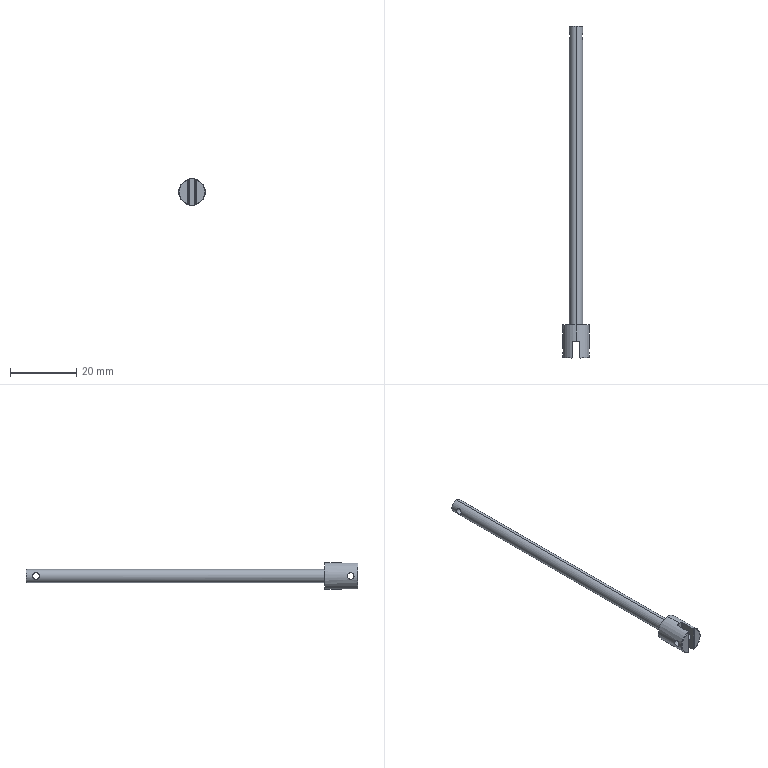Part | SolidWorks | features ICE 4, Fillet 2, Extrusion 1 | 1 solid | 23 faces | box 8 x 100 x 8 mm | volume 1520 mm3 | cylinder 14 | plane 7 | torus 2 | commonest cylinder face diameters 2 x6 0.4 x4 4 x2 8 x2
STEP:
#1=CARTESIAN_POINT('',(-1.732,-3.,1.));
#2=VERTEX_POINT('',#1);
#3=CARTESIAN_POINT('',(-1.732,-3.,-1.));
#4=VERTEX_POINT('',#3);
#5=CARTESIAN_POINT('',(-1.732,-3.,1.));
#6=CARTESIAN_POINT('',(-1.732,-3.066,1.));
#7=CARTESIAN_POINT('',(-1.736,-3.134,0.9932));
#8=CARTESIAN_POINT('',(-1.751,-3.263,0.967));
#9=CARTESIAN_POINT('',(-1.761,-3.326,0.9477));
#10=CARTESIAN_POINT('',(-1.801,-3.508,0.8713));
#11=CARTESIAN_POINT('',(-1.836,-3.616,0.798));
#12=CARTESIAN_POINT('',(-1.905,-3.798,0.6163));
#13=CARTESIAN_POINT('',(-1.939,-3.872,0.5068));
#14=CARTESIAN_POINT('',(-1.986,-3.972,0.2668));
#15=CARTESIAN_POINT('',(-2.,-4.,0.1333));
#16=CARTESIAN_POINT('',(-2.,-4.,-0.1315));
#17=CARTESIAN_POINT('',(-1.986,-3.973,-0.2649));
#18=CARTESIAN_POINT('',(-1.939,-3.872,-0.5074));
#19=CARTESIAN_POINT('',(-1.905,-3.798,-0.6164));
#20=CARTESIAN_POINT('',(-1.836,-3.615,-0.7989));
#21=CARTESIAN_POINT('',(-1.801,-3.507,-0.872));
#22=CARTESIAN_POINT('',(-1.749,-3.267,-0.9726));
#23=CARTESIAN_POINT('',(-1.732,-3.134,-1.));
#24=CARTESIAN_POINT('',(-1.732,-3.,-1.));
#25=B_SPLINE_CURVE_WITH_KNOTS('',3,(#5,#6,#7,#8,#9,#10,#11,#12,#13,#14,#15,#16,#17,#18,#19,#20,#21,#22,#23,#24),.UNSPECIFIED.,.F.,.F.,(4,2,2,2,2,2,2,2,2,4),(0.003181,0.003379,0.003577,0.003974,0.004371,0.004768,0.005165,0.005562,0.005959,0.006356),.UNSPECIFIED.);
#26=EDGE_CURVE('',#2,#4,#25,.T.);
#27=ORIENTED_EDGE('',*,*,#26,.F.);
#28=CARTESIAN_POINT('',(1.732,-3.,1.));
#29=VERTEX_POINT('',#28);
#30=CARTESIAN_POINT('',(-5.,-3.,1.));
#31=DIRECTION('',(1.,0.,0.));
#32=VECTOR('',#31,1000.);
#33=LINE('',#30,#32);
#34=EDGE_CURVE('',#2,#29,#33,.T.);
#35=ORIENTED_EDGE('',*,*,#34,.T.);
#36=CARTESIAN_POINT('',(1.732,-3.,-1.));
#37=VERTEX_POINT('',#36);
#38=CARTESIAN_POINT('',(1.732,-3.,-1.));
#39=CARTESIAN_POINT('',(1.732,-3.135,-1.));
#40=CARTESIAN_POINT('',(1.748,-3.266,-0.9727));
#41=CARTESIAN_POINT('',(1.801,-3.507,-0.8717));
#42=CARTESIAN_POINT('',(1.836,-3.616,-0.798));
#43=CARTESIAN_POINT('',(1.905,-3.798,-0.6167));
#44=CARTESIAN_POINT('',(1.938,-3.872,-0.5072));
#45=CARTESIAN_POINT('',(1.986,-3.973,-0.2669));
#46=CARTESIAN_POINT('',(2.,-4.,-0.1339));
#47=CARTESIAN_POINT('',(2.,-4.,0.1326));
#48=CARTESIAN_POINT('',(1.986,-3.973,0.2658));
#49=CARTESIAN_POINT('',(1.938,-3.871,0.5087));
#50=CARTESIAN_POINT('',(1.905,-3.797,0.6177));
#51=CARTESIAN_POINT('',(1.836,-3.615,0.7989));
#52=CARTESIAN_POINT('',(1.801,-3.506,0.8725));
#53=CARTESIAN_POINT('',(1.748,-3.266,0.9726));
#54=CARTESIAN_POINT('',(1.732,-3.133,1.));
#55=CARTESIAN_POINT('',(1.732,-3.,1.));
#56=B_SPLINE_CURVE_WITH_KNOTS('',3,(#38,#39,#40,#41,#42,#43,#44,#45,#46,#47,#48,#49,#50,#51,#52,#53,#54,#55),.UNSPECIFIED.,.F.,.F.,(4,2,2,2,2,2,2,2,4),(0.,0.0003976,0.0007951,0.001193,0.00159,0.001988,0.002385,0.002783,0.003181),.UNSPECIFIED.);
#57=EDGE_CURVE('',#37,#29,#56,.T.);
#58=ORIENTED_EDGE('',*,*,#57,.F.);
#59=CARTESIAN_POINT('',(-5.,-3.,-1.));
#60=DIRECTION('',(1.,0.,0.));
#61=VECTOR('',#60,1000.);
#62=LINE('',#59,#61);
#63=EDGE_CURVE('',#4,#37,#62,.T.);
#64=ORIENTED_EDGE('',*,*,#63,.F.);
#65=EDGE_LOOP('',(#27,#35,#58,#64));
#66=FACE_OUTER_BOUND('',#65,.T.);
#67=CARTESIAN_POINT('',(-5.,-3.,0.));
#68=DIRECTION('',(1.,0.,0.));
#69=DIRECTION('',(0.,0.,-1.));
#70=AXIS2_PLACEMENT_3D('',#67,#68,#69);
#71=CYLINDRICAL_SURFACE('',#70,1.);
#72=ADVANCED_FACE('',(#66),#71,.F.);
#73=CARTESIAN_POINT('',(-4.,-96.8,0.));
#74=VERTEX_POINT('',#73);
#75=CARTESIAN_POINT('',(-4.,-98.8,0.));
#76=VERTEX_POINT('',#75);
#77=CARTESIAN_POINT('',(-4.,-96.8,0.));
#78=CARTESIAN_POINT('',(-4.,-96.8,-0.1327));
#79=CARTESIAN_POINT('',(-3.993,-96.826,-0.2629));
#80=CARTESIAN_POINT('',(-3.97,-96.927,-0.5049));
#81=CARTESIAN_POINT('',(-3.953,-97.001,-0.6155));
#82=CARTESIAN_POINT('',(-3.92,-97.185,-0.7991));
#83=CARTESIAN_POINT('',(-3.904,-97.296,-0.8735));
#84=CARTESIAN_POINT('',(-3.88,-97.537,-0.9734));
#85=CARTESIAN_POINT('',(-3.873,-97.669,-0.9999));
#86=CARTESIAN_POINT('',(-3.873,-97.931,-1.));
#87=CARTESIAN_POINT('',(-3.88,-98.062,-0.974));
#88=CARTESIAN_POINT('',(-3.904,-98.305,-0.8732));
#89=CARTESIAN_POINT('',(-3.92,-98.415,-0.7996));
#90=CARTESIAN_POINT('',(-3.954,-98.6,-0.6143));
#91=CARTESIAN_POINT('',(-3.97,-98.673,-0.5041));
#92=CARTESIAN_POINT('',(-3.993,-98.774,-0.2626));
#93=CARTESIAN_POINT('',(-4.,-98.8,-0.1308));
#94=CARTESIAN_POINT('',(-4.,-98.8,0.));
#95=B_SPLINE_CURVE_WITH_KNOTS('',3,(#77,#78,#79,#80,#81,#82,#83,#84,#85,#86,#87,#88,#89,#90,#91,#92,#93,#94),.UNSPECIFIED.,.F.,.F.,(4,2,2,2,2,2,2,2,4),(0.,0.0003924,0.0007847,0.001177,0.001569,0.001962,0.002354,0.002747,0.003139),.UNSPECIFIED.);
#96=EDGE_CURVE('',#74,#76,#95,.T.);
#97=ORIENTED_EDGE('',*,*,#96,.T.);
#98=CARTESIAN_POINT('',(-1.05,-98.8,0.));
#99=VERTEX_POINT('',#98);
#100=CARTESIAN_POINT('',(-201.05,-98.8,0.));
#101=DIRECTION('',(1.,0.,0.));
#102=VECTOR('',#101,1000.);
#103=LINE('',#100,#102);
#104=EDGE_CURVE('',#76,#99,#103,.T.);
#105=ORIENTED_EDGE('',*,*,#104,.T.);
#106=CARTESIAN_POINT('',(-1.05,-96.8,0.));
#107=VERTEX_POINT('',#106);
#108=CARTESIAN_POINT('',(-1.05,-97.8,0.));
#109=DIRECTION('',(-1.,0.,0.));
#110=DIRECTION('',(0.,-1.,0.));
#111=AXIS2_PLACEMENT_3D('',#108,#109,#110);
#112=CIRCLE('',#111,1.);
#113=EDGE_CURVE('',#107,#99,#112,.T.);
#114=ORIENTED_EDGE('',*,*,#113,.F.);
#115=CARTESIAN_POINT('',(-201.05,-96.8,0.));
#116=DIRECTION('',(1.,0.,0.));
#117=VECTOR('',#116,1000.);
#118=LINE('',#115,#117);
#119=EDGE_CURVE('',#74,#107,#118,.T.);
#120=ORIENTED_EDGE('',*,*,#119,.F.);
#121=EDGE_LOOP('',(#97,#105,#114,#120));
#122=FACE_OUTER_BOUND('',#121,.T.);
#123=CARTESIAN_POINT('',(-201.05,-97.8,0.));
#124=DIRECTION('',(1.,0.,0.));
#125=DIRECTION('',(0.,1.,0.));
#126=AXIS2_PLACEMENT_3D('',#123,#124,#125);
#127=CYLINDRICAL_SURFACE('',#126,1.);
#128=ADVANCED_FACE('',(#122),#127,.F.);
#129=CARTESIAN_POINT('',(1.05,-98.8,0.));
#130=VERTEX_POINT('',#129);
#131=CARTESIAN_POINT('',(1.05,-96.8,0.));
#132=VERTEX_POINT('',#131);
#133=CARTESIAN_POINT('',(1.05,-97.8,0.));
#134=DIRECTION('',(1.,0.,0.));
#135=DIRECTION('',(0.,1.,0.));
#136=AXIS2_PLACEMENT_3D('',#133,#134,#135);
#137=CIRCLE('',#136,1.);
#138=EDGE_CURVE('',#130,#132,#137,.T.);
#139=ORIENTED_EDGE('',*,*,#138,.F.);
#140=CARTESIAN_POINT('',(4.,-98.8,0.));
#141=VERTEX_POINT('',#140);
#142=CARTESIAN_POINT('',(-201.05,-98.8,0.));
#143=DIRECTION('',(1.,0.,0.));
#144=VECTOR('',#143,1000.);
#145=LINE('',#142,#144);
#146=EDGE_CURVE('',#130,#141,#145,.T.);
#147=ORIENTED_EDGE('',*,*,#146,.T.);
#148=CARTESIAN_POINT('',(4.,-96.8,0.));
#149=VERTEX_POINT('',#148);
#150=CARTESIAN_POINT('',(4.,-98.8,0.));
#151=CARTESIAN_POINT('',(4.,-98.8,-0.1308));
#152=CARTESIAN_POINT('',(3.993,-98.774,-0.2629));
#153=CARTESIAN_POINT('',(3.97,-98.674,-0.5038));
#154=CARTESIAN_POINT('',(3.954,-98.6,-0.6146));
#155=CARTESIAN_POINT('',(3.92,-98.415,-0.7991));
#156=CARTESIAN_POINT('',(3.904,-98.306,-0.8727));
#157=CARTESIAN_POINT('',(3.88,-98.062,-0.9739));
#158=CARTESIAN_POINT('',(3.873,-97.932,-1.));
#159=CARTESIAN_POINT('',(3.873,-97.668,-1.));
#160=CARTESIAN_POINT('',(3.88,-97.537,-0.9737));
#161=CARTESIAN_POINT('',(3.904,-97.296,-0.8736));
#162=CARTESIAN_POINT('',(3.92,-97.185,-0.7992));
#163=CARTESIAN_POINT('',(3.953,-97.001,-0.6158));
#164=CARTESIAN_POINT('',(3.97,-96.927,-0.5048));
#165=CARTESIAN_POINT('',(3.993,-96.827,-0.2641));
#166=CARTESIAN_POINT('',(4.,-96.8,-0.1327));
#167=CARTESIAN_POINT('',(4.,-96.8,0.));
#168=B_SPLINE_CURVE_WITH_KNOTS('',3,(#150,#151,#152,#153,#154,#155,#156,#157,#158,#159,#160,#161,#162,#163,#164,#165,#166,#167),.UNSPECIFIED.,.F.,.F.,(4,2,2,2,2,2,2,2,4),(0.003139,0.003531,0.003923,0.004316,0.004708,0.0051,0.005493,0.005885,0.006277),.UNSPECIFIED.);
#169=EDGE_CURVE('',#141,#149,#168,.T.);
#170=ORIENTED_EDGE('',*,*,#169,.T.);
#171=CARTESIAN_POINT('',(-201.05,-96.8,0.));
#172=DIRECTION('',(1.,0.,0.));
#173=VECTOR('',#172,1000.);
#174=LINE('',#171,#173);
#175=EDGE_CURVE('',#132,#149,#174,.T.);
#176=ORIENTED_EDGE('',*,*,#175,.F.);
#177=EDGE_LOOP('',(#139,#147,#170,#176));
#178=FACE_OUTER_BOUND('',#177,.T.);
#179=CARTESIAN_POINT('',(-201.05,-97.8,0.));
#180=DIRECTION('',(1.,0.,0.));
#181=DIRECTION('',(0.,1.,0.));
#182=AXIS2_PLACEMENT_3D('',#179,#180,#181);
#183=CYLINDRICAL_SURFACE('',#182,1.);
#184=ADVANCED_FACE('',(#178),#183,.F.);
#185=CARTESIAN_POINT('',(4.,-96.8,0.));
#186=CARTESIAN_POINT('',(4.,-96.8,0.1327));
#187=CARTESIAN_POINT('',(3.993,-96.826,0.2629));
#188=CARTESIAN_POINT('',(3.97,-96.927,0.5049));
#189=CARTESIAN_POINT('',(3.953,-97.001,0.6155));
#190=CARTESIAN_POINT('',(3.92,-97.185,0.7991));
#191=CARTESIAN_POINT('',(3.904,-97.296,0.8735));
#192=CARTESIAN_POINT('',(3.88,-97.537,0.9734));
#193=CARTESIAN_POINT('',(3.873,-97.669,0.9999));
#194=CARTESIAN_POINT('',(3.873,-97.931,1.));
#195=CARTESIAN_POINT('',(3.88,-98.062,0.974));
#196=CARTESIAN_POINT('',(3.904,-98.305,0.8732));
#197=CARTESIAN_POINT('',(3.92,-98.415,0.7996));
#198=CARTESIAN_POINT('',(3.954,-98.6,0.6143));
#199=CARTESIAN_POINT('',(3.97,-98.673,0.5041));
#200=CARTESIAN_POINT('',(3.993,-98.774,0.2626));
#201=CARTESIAN_POINT('',(4.,-98.8,0.1308));
#202=CARTESIAN_POINT('',(4.,-98.8,0.));
#203=B_SPLINE_CURVE_WITH_KNOTS('',3,(#185,#186,#187,#188,#189,#190,#191,#192,#193,#194,#195,#196,#197,#198,#199,#200,#201,#202),.UNSPECIFIED.,.F.,.F.,(4,2,2,2,2,2,2,2,4),(0.,0.0003924,0.0007847,0.001177,0.001569,0.001962,0.002354,0.002747,0.003139),.UNSPECIFIED.);
#204=EDGE_CURVE('',#149,#141,#203,.T.);
#205=ORIENTED_EDGE('',*,*,#204,.F.);
#206=ORIENTED_EDGE('',*,*,#169,.F.);
#207=EDGE_LOOP('',(#205,#206));
#208=FACE_BOUND('',#207,.T.);
#209=CARTESIAN_POINT('',(0.,-90.,-4.));
#210=VERTEX_POINT('',#209);
#211=CARTESIAN_POINT('',(0.,-90.,4.));
#212=VERTEX_POINT('',#211);
#213=CARTESIAN_POINT('',(0.,-90.,0.));
#214=DIRECTION('',(0.,-1.,0.));
#215=DIRECTION('',(0.,0.,-1.));
#216=AXIS2_PLACEMENT_3D('',#213,#214,#215);
#217=CIRCLE('',#216,4.);
#218=EDGE_CURVE('',#210,#212,#217,.T.);
#219=ORIENTED_EDGE('',*,*,#218,.T.);
#220=CARTESIAN_POINT('',(0.,-95.,4.));
#221=VERTEX_POINT('',#220);
#222=CARTESIAN_POINT('',(0.,-90.,4.));
#223=DIRECTION('',(0.,-1.,0.));
#224=VECTOR('',#223,1000.);
#225=LINE('',#222,#224);
#226=EDGE_CURVE('',#212,#221,#225,.T.);
#227=ORIENTED_EDGE('',*,*,#226,.T.);
#228=CARTESIAN_POINT('',(0.85,-95.,3.909));
#229=VERTEX_POINT('',#228);
#230=CARTESIAN_POINT('',(0.,-95.,0.));
#231=DIRECTION('',(0.,-1.,0.));
#232=DIRECTION('',(0.,0.,1.));
#233=AXIS2_PLACEMENT_3D('',#230,#231,#232);
#234=CIRCLE('',#233,4.);
#235=EDGE_CURVE('',#229,#221,#234,.T.);
#236=ORIENTED_EDGE('',*,*,#235,.F.);
#237=CARTESIAN_POINT('',(1.05,-95.2,3.86));
#238=VERTEX_POINT('',#237);
#239=CARTESIAN_POINT('',(0.85,-95.,3.909));
#240=CARTESIAN_POINT('',(0.9024,-95.,3.897));
#241=CARTESIAN_POINT('',(0.9534,-95.021,3.885));
#242=CARTESIAN_POINT('',(1.028,-95.094,3.866));
#243=CARTESIAN_POINT('',(1.05,-95.146,3.86));
#244=CARTESIAN_POINT('',(1.05,-95.2,3.86));
#245=B_SPLINE_CURVE_WITH_KNOTS('',3,(#239,#240,#241,#242,#243,#244),.UNSPECIFIED.,.F.,.F.,(4,2,4),(0.,0.0001585,0.0003169),.UNSPECIFIED.);
#246=EDGE_CURVE('',#229,#238,#245,.T.);
#247=ORIENTED_EDGE('',*,*,#246,.T.);
#248=CARTESIAN_POINT('',(1.05,-99.8,3.86));
#249=VERTEX_POINT('',#248);
#250=CARTESIAN_POINT('',(1.05,-90.,3.86));
#251=DIRECTION('',(0.,1.,0.));
#252=VECTOR('',#251,1000.);
#253=LINE('',#250,#252);
#254=EDGE_CURVE('',#249,#238,#253,.T.);
#255=ORIENTED_EDGE('',*,*,#254,.F.);
#256=CARTESIAN_POINT('',(1.05,-99.8,-3.86));
#257=VERTEX_POINT('',#256);
#258=CARTESIAN_POINT('',(0.,-99.8,0.));
#259=DIRECTION('',(0.,1.,0.));
#260=DIRECTION('',(0.,0.,-1.));
#261=AXIS2_PLACEMENT_3D('',#258,#259,#260);
#262=CIRCLE('',#261,4.);
#263=EDGE_CURVE('',#249,#257,#262,.T.);
#264=ORIENTED_EDGE('',*,*,#263,.T.);
#265=CARTESIAN_POINT('',(1.05,-95.2,-3.86));
#266=VERTEX_POINT('',#265);
#267=CARTESIAN_POINT('',(1.05,-90.,-3.86));
#268=DIRECTION('',(0.,-1.,0.));
#269=VECTOR('',#268,1000.);
#270=LINE('',#267,#269);
#271=EDGE_CURVE('',#266,#257,#270,.T.);
#272=ORIENTED_EDGE('',*,*,#271,.F.);
#273=CARTESIAN_POINT('',(0.85,-95.,-3.909));
#274=VERTEX_POINT('',#273);
#275=CARTESIAN_POINT('',(1.05,-95.2,-3.86));
#276=CARTESIAN_POINT('',(1.05,-95.146,-3.86));
#277=CARTESIAN_POINT('',(1.028,-95.094,-3.866));
#278=CARTESIAN_POINT('',(0.9536,-95.021,-3.885));
#279=CARTESIAN_POINT('',(0.9023,-95.,-3.897));
#280=CARTESIAN_POINT('',(0.85,-95.,-3.909));
#281=B_SPLINE_CURVE_WITH_KNOTS('',3,(#275,#276,#277,#278,#279,#280),.UNSPECIFIED.,.F.,.F.,(4,2,4),(0.,0.0001585,0.0003169),.UNSPECIFIED.);
#282=EDGE_CURVE('',#266,#274,#281,.T.);
#283=ORIENTED_EDGE('',*,*,#282,.T.);
#284=CARTESIAN_POINT('',(0.,-95.,-4.));
#285=VERTEX_POINT('',#284);
#286=CARTESIAN_POINT('',(0.,-95.,0.));
#287=DIRECTION('',(0.,-1.,0.));
#288=DIRECTION('',(0.,0.,1.));
#289=AXIS2_PLACEMENT_3D('',#286,#287,#288);
#290=CIRCLE('',#289,4.);
#291=EDGE_CURVE('',#285,#274,#290,.T.);
#292=ORIENTED_EDGE('',*,*,#291,.F.);
#293=CARTESIAN_POINT('',(0.,-90.,-4.));
#294=DIRECTION('',(0.,-1.,0.));
#295=VECTOR('',#294,1000.);
#296=LINE('',#293,#295);
#297=EDGE_CURVE('',#210,#285,#296,.T.);
#298=ORIENTED_EDGE('',*,*,#297,.F.);
#299=EDGE_LOOP('',(#219,#227,#236,#247,#255,#264,#272,#283,#292,#298));
#300=FACE_OUTER_BOUND('',#299,.T.);
#301=CARTESIAN_POINT('',(0.,-90.,0.));
#302=DIRECTION('',(0.,-1.,0.));
#303=DIRECTION('',(0.,0.,-1.));
#304=AXIS2_PLACEMENT_3D('',#301,#302,#303);
#305=CYLINDRICAL_SURFACE('',#304,4.);
#306=ADVANCED_FACE('',(#208,#300),#305,.T.);
#307=ORIENTED_EDGE('',*,*,#57,.T.);
#308=CARTESIAN_POINT('',(1.732,-3.,1.));
#309=CARTESIAN_POINT('',(1.732,-2.934,1.));
#310=CARTESIAN_POINT('',(1.736,-2.866,0.9932));
#311=CARTESIAN_POINT('',(1.751,-2.737,0.967));
#312=CARTESIAN_POINT('',(1.761,-2.674,0.9477));
#313=CARTESIAN_POINT('',(1.801,-2.492,0.8713));
#314=CARTESIAN_POINT('',(1.836,-2.384,0.798));
#315=CARTESIAN_POINT('',(1.905,-2.202,0.6163));
#316=CARTESIAN_POINT('',(1.939,-2.128,0.5068));
#317=CARTESIAN_POINT('',(1.986,-2.028,0.2668));
#318=CARTESIAN_POINT('',(2.,-2.,0.1333));
#319=CARTESIAN_POINT('',(2.,-2.,-0.1315));
#320=CARTESIAN_POINT('',(1.986,-2.027,-0.2649));
#321=CARTESIAN_POINT('',(1.939,-2.128,-0.5074));
#322=CARTESIAN_POINT('',(1.905,-2.202,-0.6164));
#323=CARTESIAN_POINT('',(1.836,-2.385,-0.7989));
#324=CARTESIAN_POINT('',(1.801,-2.493,-0.872));
#325=CARTESIAN_POINT('',(1.749,-2.733,-0.9726));
#326=CARTESIAN_POINT('',(1.732,-2.866,-1.));
#327=CARTESIAN_POINT('',(1.732,-3.,-1.));
#328=B_SPLINE_CURVE_WITH_KNOTS('',3,(#308,#309,#310,#311,#312,#313,#314,#315,#316,#317,#318,#319,#320,#321,#322,#323,#324,#325,#326,#327),.UNSPECIFIED.,.F.,.F.,(4,2,2,2,2,2,2,2,2,4),(0.003181,0.003379,0.003577,0.003974,0.004371,0.004768,0.005165,0.005562,0.005959,0.006356),.UNSPECIFIED.);
#329=EDGE_CURVE('',#29,#37,#328,.T.);
#330=ORIENTED_EDGE('',*,*,#329,.T.);
#331=EDGE_LOOP('',(#307,#330));
#332=FACE_BOUND('',#331,.T.);
#333=CARTESIAN_POINT('',(0.,-90.,-2.));
#334=VERTEX_POINT('',#333);
#335=CARTESIAN_POINT('',(0.,-90.,2.));
#336=VERTEX_POINT('',#335);
#337=CARTESIAN_POINT('',(0.,-90.,0.));
#338=DIRECTION('',(0.,-1.,0.));
#339=DIRECTION('',(0.,0.,-1.));
#340=AXIS2_PLACEMENT_3D('',#337,#338,#339);
#341=CIRCLE('',#340,2.);
#342=EDGE_CURVE('',#334,#336,#341,.T.);
#343=ORIENTED_EDGE('',*,*,#342,.F.);
#344=CARTESIAN_POINT('',(0.,0.,-2.));
#345=VERTEX_POINT('',#344);
#346=CARTESIAN_POINT('',(0.,-100.,-2.));
#347=DIRECTION('',(0.,1.,0.));
#348=VECTOR('',#347,1000.);
#349=LINE('',#346,#348);
#350=EDGE_CURVE('',#334,#345,#349,.T.);
#351=ORIENTED_EDGE('',*,*,#350,.T.);
#352=CARTESIAN_POINT('',(0.,0.,2.));
#353=VERTEX_POINT('',#352);
#354=CARTESIAN_POINT('',(0.,0.,0.));
#355=DIRECTION('',(0.,-1.,0.));
#356=DIRECTION('',(0.,0.,-1.));
#357=AXIS2_PLACEMENT_3D('',#354,#355,#356);
#358=CIRCLE('',#357,2.);
#359=EDGE_CURVE('',#345,#353,#358,.T.);
#360=ORIENTED_EDGE('',*,*,#359,.T.);
#361=CARTESIAN_POINT('',(0.,-100.,2.));
#362=DIRECTION('',(0.,1.,0.));
#363=VECTOR('',#362,1000.);
#364=LINE('',#361,#363);
#365=EDGE_CURVE('',#336,#353,#364,.T.);
#366=ORIENTED_EDGE('',*,*,#365,.F.);
#367=EDGE_LOOP('',(#343,#351,#360,#366));
#368=FACE_OUTER_BOUND('',#367,.T.);
#369=CARTESIAN_POINT('',(0.,-100.,0.));
#370=DIRECTION('',(0.,1.,0.));
#371=DIRECTION('',(0.,0.,1.));
#372=AXIS2_PLACEMENT_3D('',#369,#370,#371);
#373=CYLINDRICAL_SURFACE('',#372,2.);
#374=ADVANCED_FACE('',(#332,#368),#373,.T.);
#375=CARTESIAN_POINT('',(-1.25,-100.,-3.589));
#376=VERTEX_POINT('',#375);
#377=CARTESIAN_POINT('',(-1.25,-100.,3.589));
#378=VERTEX_POINT('',#377);
#379=CARTESIAN_POINT('',(-1.25,-100.,3.86));
#380=DIRECTION('',(0.,0.,1.));
#381=VECTOR('',#380,1000.);
#382=LINE('',#379,#381);
#383=EDGE_CURVE('',#376,#378,#382,.T.);
#384=ORIENTED_EDGE('',*,*,#383,.T.);
#385=CARTESIAN_POINT('',(0.,-100.,0.));
#386=DIRECTION('',(0.,-1.,0.));
#387=DIRECTION('',(0.,0.,-1.));
#388=AXIS2_PLACEMENT_3D('',#385,#386,#387);
#389=CIRCLE('',#388,3.8);
#390=EDGE_CURVE('',#378,#376,#389,.T.);
#391=ORIENTED_EDGE('',*,*,#390,.T.);
#392=EDGE_LOOP('',(#384,#391));
#393=FACE_OUTER_BOUND('',#392,.T.);
#394=CARTESIAN_POINT('',(0.,-100.,0.));
#395=DIRECTION('',(0.,-1.,0.));
#396=DIRECTION('',(0.,0.,-1.));
#397=AXIS2_PLACEMENT_3D('',#394,#395,#396);
#398=PLANE('',#397);
#399=ADVANCED_FACE('',(#393),#398,.T.);
#400=ORIENTED_EDGE('',*,*,#350,.F.);
#401=CARTESIAN_POINT('',(0.,-90.,0.));
#402=DIRECTION('',(0.,-1.,0.));
#403=DIRECTION('',(0.,0.,-1.));
#404=AXIS2_PLACEMENT_3D('',#401,#402,#403);
#405=CIRCLE('',#404,2.);
#406=EDGE_CURVE('',#336,#334,#405,.T.);
#407=ORIENTED_EDGE('',*,*,#406,.F.);
#408=ORIENTED_EDGE('',*,*,#365,.T.);
#409=CARTESIAN_POINT('',(0.,0.,0.));
#410=DIRECTION('',(0.,-1.,0.));
#411=DIRECTION('',(0.,0.,-1.));
#412=AXIS2_PLACEMENT_3D('',#409,#410,#411);
#413=CIRCLE('',#412,2.);
#414=EDGE_CURVE('',#353,#345,#413,.T.);
#415=ORIENTED_EDGE('',*,*,#414,.T.);
#416=EDGE_LOOP('',(#400,#407,#408,#415));
#417=FACE_OUTER_BOUND('',#416,.T.);
#418=CARTESIAN_POINT('',(-1.732,-3.,-1.));
#419=CARTESIAN_POINT('',(-1.732,-2.865,-1.));
#420=CARTESIAN_POINT('',(-1.748,-2.734,-0.9727));
#421=CARTESIAN_POINT('',(-1.801,-2.493,-0.8717));
#422=CARTESIAN_POINT('',(-1.836,-2.384,-0.798));
#423=CARTESIAN_POINT('',(-1.905,-2.202,-0.6167));
#424=CARTESIAN_POINT('',(-1.938,-2.128,-0.5072));
#425=CARTESIAN_POINT('',(-1.986,-2.027,-0.2669));
#426=CARTESIAN_POINT('',(-2.,-2.,-0.1339));
#427=CARTESIAN_POINT('',(-2.,-2.,0.1326));
#428=CARTESIAN_POINT('',(-1.986,-2.027,0.2658));
#429=CARTESIAN_POINT('',(-1.938,-2.129,0.5087));
#430=CARTESIAN_POINT('',(-1.905,-2.203,0.6177));
#431=CARTESIAN_POINT('',(-1.836,-2.385,0.7989));
#432=CARTESIAN_POINT('',(-1.801,-2.494,0.8725));
#433=CARTESIAN_POINT('',(-1.748,-2.734,0.9726));
#434=CARTESIAN_POINT('',(-1.732,-2.867,1.));
#435=CARTESIAN_POINT('',(-1.732,-3.,1.));
#436=B_SPLINE_CURVE_WITH_KNOTS('',3,(#418,#419,#420,#421,#422,#423,#424,#425,#426,#427,#428,#429,#430,#431,#432,#433,#434,#435),.UNSPECIFIED.,.F.,.F.,(4,2,2,2,2,2,2,2,4),(0.,0.0003976,0.0007951,0.001193,0.00159,0.001988,0.002385,0.002783,0.003181),.UNSPECIFIED.);
#437=EDGE_CURVE('',#4,#2,#436,.T.);
#438=ORIENTED_EDGE('',*,*,#437,.T.);
#439=ORIENTED_EDGE('',*,*,#26,.T.);
#440=EDGE_LOOP('',(#438,#439));
#441=FACE_BOUND('',#440,.T.);
#442=CARTESIAN_POINT('',(0.,-100.,0.));
#443=DIRECTION('',(0.,1.,0.));
#444=DIRECTION('',(0.,0.,1.));
#445=AXIS2_PLACEMENT_3D('',#442,#443,#444);
#446=CYLINDRICAL_SURFACE('',#445,2.);
#447=ADVANCED_FACE('',(#417,#441),#446,.T.);
#448=ORIENTED_EDGE('',*,*,#414,.F.);
#449=ORIENTED_EDGE('',*,*,#359,.F.);
#450=EDGE_LOOP('',(#448,#449));
#451=FACE_OUTER_BOUND('',#450,.T.);
#452=CARTESIAN_POINT('',(0.,0.,0.));
#453=DIRECTION('',(0.,-1.,0.));
#454=DIRECTION('',(0.,0.,-1.));
#455=AXIS2_PLACEMENT_3D('',#452,#453,#454);
#456=PLANE('',#455);
#457=ADVANCED_FACE('',(#451),#456,.F.);
#458=ORIENTED_EDGE('',*,*,#226,.F.);
#459=CARTESIAN_POINT('',(0.,-90.,0.));
#460=DIRECTION('',(0.,-1.,0.));
#461=DIRECTION('',(0.,0.,-1.));
#462=AXIS2_PLACEMENT_3D('',#459,#460,#461);
#463=CIRCLE('',#462,4.);
#464=EDGE_CURVE('',#212,#210,#463,.T.);
#465=ORIENTED_EDGE('',*,*,#464,.T.);
#466=ORIENTED_EDGE('',*,*,#297,.T.);
#467=CARTESIAN_POINT('',(-0.85,-95.,-3.909));
#468=VERTEX_POINT('',#467);
#469=CARTESIAN_POINT('',(0.,-95.,0.));
#470=DIRECTION('',(0.,-1.,0.));
#471=DIRECTION('',(0.,0.,1.));
#472=AXIS2_PLACEMENT_3D('',#469,#470,#471);
#473=CIRCLE('',#472,4.);
#474=EDGE_CURVE('',#468,#285,#473,.T.);
#475=ORIENTED_EDGE('',*,*,#474,.F.);
#476=CARTESIAN_POINT('',(-1.05,-95.2,-3.86));
#477=VERTEX_POINT('',#476);
#478=CARTESIAN_POINT('',(-0.85,-95.,-3.909));
#479=CARTESIAN_POINT('',(-0.9024,-95.,-3.897));
#480=CARTESIAN_POINT('',(-0.9534,-95.021,-3.885));
#481=CARTESIAN_POINT('',(-1.028,-95.094,-3.866));
#482=CARTESIAN_POINT('',(-1.05,-95.146,-3.86));
#483=CARTESIAN_POINT('',(-1.05,-95.2,-3.86));
#484=B_SPLINE_CURVE_WITH_KNOTS('',3,(#478,#479,#480,#481,#482,#483),.UNSPECIFIED.,.F.,.F.,(4,2,4),(0.,0.0001585,0.0003169),.UNSPECIFIED.);
#485=EDGE_CURVE('',#468,#477,#484,.T.);
#486=ORIENTED_EDGE('',*,*,#485,.T.);
#487=CARTESIAN_POINT('',(-1.05,-99.8,-3.86));
#488=VERTEX_POINT('',#487);
#489=CARTESIAN_POINT('',(-1.05,-90.,-3.86));
#490=DIRECTION('',(0.,1.,0.));
#491=VECTOR('',#490,1000.);
#492=LINE('',#489,#491);
#493=EDGE_CURVE('',#488,#477,#492,.T.);
#494=ORIENTED_EDGE('',*,*,#493,.F.);
#495=CARTESIAN_POINT('',(-1.05,-99.8,3.86));
#496=VERTEX_POINT('',#495);
#497=CARTESIAN_POINT('',(0.,-99.8,0.));
#498=DIRECTION('',(0.,1.,0.));
#499=DIRECTION('',(0.,0.,-1.));
#500=AXIS2_PLACEMENT_3D('',#497,#498,#499);
#501=CIRCLE('',#500,4.);
#502=EDGE_CURVE('',#488,#496,#501,.T.);
#503=ORIENTED_EDGE('',*,*,#502,.T.);
#504=CARTESIAN_POINT('',(-1.05,-95.2,3.86));
#505=VERTEX_POINT('',#504);
#506=CARTESIAN_POINT('',(-1.05,-90.,3.86));
#507=DIRECTION('',(0.,-1.,0.));
#508=VECTOR('',#507,1000.);
#509=LINE('',#506,#508);
#510=EDGE_CURVE('',#505,#496,#509,.T.);
#511=ORIENTED_EDGE('',*,*,#510,.F.);
#512=CARTESIAN_POINT('',(-0.85,-95.,3.909));
#513=VERTEX_POINT('',#512);
#514=CARTESIAN_POINT('',(-1.05,-95.2,3.86));
#515=CARTESIAN_POINT('',(-1.05,-95.146,3.86));
#516=CARTESIAN_POINT('',(-1.028,-95.094,3.866));
#517=CARTESIAN_POINT('',(-0.9536,-95.021,3.885));
#518=CARTESIAN_POINT('',(-0.9023,-95.,3.897));
#519=CARTESIAN_POINT('',(-0.85,-95.,3.909));
#520=B_SPLINE_CURVE_WITH_KNOTS('',3,(#514,#515,#516,#517,#518,#519),.UNSPECIFIED.,.F.,.F.,(4,2,4),(0.,0.0001585,0.0003169),.UNSPECIFIED.);
#521=EDGE_CURVE('',#505,#513,#520,.T.);
#522=ORIENTED_EDGE('',*,*,#521,.T.);
#523=CARTESIAN_POINT('',(0.,-95.,0.));
#524=DIRECTION('',(0.,-1.,0.));
#525=DIRECTION('',(0.,0.,1.));
#526=AXIS2_PLACEMENT_3D('',#523,#524,#525);
#527=CIRCLE('',#526,4.);
#528=EDGE_CURVE('',#221,#513,#527,.T.);
#529=ORIENTED_EDGE('',*,*,#528,.F.);
#530=EDGE_LOOP('',(#458,#465,#466,#475,#486,#494,#503,#511,#522,#529));
#531=FACE_OUTER_BOUND('',#530,.T.);
#532=ORIENTED_EDGE('',*,*,#96,.F.);
#533=CARTESIAN_POINT('',(-4.,-98.8,0.));
#534=CARTESIAN_POINT('',(-4.,-98.8,0.1308));
#535=CARTESIAN_POINT('',(-3.993,-98.774,0.2629));
#536=CARTESIAN_POINT('',(-3.97,-98.674,0.5038));
#537=CARTESIAN_POINT('',(-3.954,-98.6,0.6146));
#538=CARTESIAN_POINT('',(-3.92,-98.415,0.7991));
#539=CARTESIAN_POINT('',(-3.904,-98.306,0.8727));
#540=CARTESIAN_POINT('',(-3.88,-98.062,0.9739));
#541=CARTESIAN_POINT('',(-3.873,-97.932,1.));
#542=CARTESIAN_POINT('',(-3.873,-97.668,1.));
#543=CARTESIAN_POINT('',(-3.88,-97.537,0.9737));
#544=CARTESIAN_POINT('',(-3.904,-97.296,0.8736));
#545=CARTESIAN_POINT('',(-3.92,-97.185,0.7992));
#546=CARTESIAN_POINT('',(-3.953,-97.001,0.6158));
#547=CARTESIAN_POINT('',(-3.97,-96.927,0.5048));
#548=CARTESIAN_POINT('',(-3.993,-96.827,0.2641));
#549=CARTESIAN_POINT('',(-4.,-96.8,0.1327));
#550=CARTESIAN_POINT('',(-4.,-96.8,0.));
#551=B_SPLINE_CURVE_WITH_KNOTS('',3,(#533,#534,#535,#536,#537,#538,#539,#540,#541,#542,#543,#544,#545,#546,#547,#548,#549,#550),.UNSPECIFIED.,.F.,.F.,(4,2,2,2,2,2,2,2,4),(0.003139,0.003531,0.003923,0.004316,0.004708,0.0051,0.005493,0.005885,0.006277),.UNSPECIFIED.);
#552=EDGE_CURVE('',#76,#74,#551,.T.);
#553=ORIENTED_EDGE('',*,*,#552,.F.);
#554=EDGE_LOOP('',(#532,#553));
#555=FACE_BOUND('',#554,.T.);
#556=CARTESIAN_POINT('',(0.,-90.,0.));
#557=DIRECTION('',(0.,-1.,0.));
#558=DIRECTION('',(0.,0.,-1.));
#559=AXIS2_PLACEMENT_3D('',#556,#557,#558);
#560=CYLINDRICAL_SURFACE('',#559,4.);
#561=ADVANCED_FACE('',(#531,#555),#560,.T.);
#562=ORIENTED_EDGE('',*,*,#406,.T.);
#563=ORIENTED_EDGE('',*,*,#342,.T.);
#564=EDGE_LOOP('',(#562,#563));
#565=FACE_BOUND('',#564,.T.);
#566=ORIENTED_EDGE('',*,*,#218,.F.);
#567=ORIENTED_EDGE('',*,*,#464,.F.);
#568=EDGE_LOOP('',(#566,#567));
#569=FACE_OUTER_BOUND('',#568,.T.);
#570=CARTESIAN_POINT('',(0.,-90.,0.));
#571=DIRECTION('',(0.,-1.,0.));
#572=DIRECTION('',(0.,0.,-1.));
#573=AXIS2_PLACEMENT_3D('',#570,#571,#572);
#574=PLANE('',#573);
#575=ADVANCED_FACE('',(#565,#569),#574,.F.);
#576=CARTESIAN_POINT('',(1.25,-100.,3.589));
#577=VERTEX_POINT('',#576);
#578=CARTESIAN_POINT('',(1.25,-100.,-3.589));
#579=VERTEX_POINT('',#578);
#580=CARTESIAN_POINT('',(1.25,-100.,-3.86));
#581=DIRECTION('',(0.,0.,-1.));
#582=VECTOR('',#581,1000.);
#583=LINE('',#580,#582);
#584=EDGE_CURVE('',#577,#579,#583,.T.);
#585=ORIENTED_EDGE('',*,*,#584,.T.);
#586=CARTESIAN_POINT('',(0.,-100.,0.));
#587=DIRECTION('',(0.,-1.,0.));
#588=DIRECTION('',(0.,0.,-1.));
#589=AXIS2_PLACEMENT_3D('',#586,#587,#588);
#590=CIRCLE('',#589,3.8);
#591=EDGE_CURVE('',#579,#577,#590,.T.);
#592=ORIENTED_EDGE('',*,*,#591,.T.);
#593=EDGE_LOOP('',(#585,#592));
#594=FACE_OUTER_BOUND('',#593,.T.);
#595=CARTESIAN_POINT('',(0.,-100.,0.));
#596=DIRECTION('',(0.,-1.,0.));
#597=DIRECTION('',(0.,0.,-1.));
#598=AXIS2_PLACEMENT_3D('',#595,#596,#597);
#599=PLANE('',#598);
#600=ADVANCED_FACE('',(#594),#599,.T.);
#601=ORIENTED_EDGE('',*,*,#113,.T.);
#602=CARTESIAN_POINT('',(-1.05,-97.8,0.));
#603=DIRECTION('',(-1.,0.,0.));
#604=DIRECTION('',(0.,-1.,0.));
#605=AXIS2_PLACEMENT_3D('',#602,#603,#604);
#606=CIRCLE('',#605,1.);
#607=EDGE_CURVE('',#99,#107,#606,.T.);
#608=ORIENTED_EDGE('',*,*,#607,.T.);
#609=EDGE_LOOP('',(#601,#608));
#610=FACE_BOUND('',#609,.T.);
#611=ORIENTED_EDGE('',*,*,#493,.T.);
#612=CARTESIAN_POINT('',(-1.05,-95.2,3.86));
#613=DIRECTION('',(0.,0.,1.));
#614=VECTOR('',#613,1000.);
#615=LINE('',#612,#614);
#616=EDGE_CURVE('',#477,#505,#615,.T.);
#617=ORIENTED_EDGE('',*,*,#616,.T.);
#618=ORIENTED_EDGE('',*,*,#510,.T.);
#619=CARTESIAN_POINT('',(-1.05,-99.8,-3.86));
#620=DIRECTION('',(0.,0.,-1.));
#621=VECTOR('',#620,1000.);
#622=LINE('',#619,#621);
#623=EDGE_CURVE('',#496,#488,#622,.T.);
#624=ORIENTED_EDGE('',*,*,#623,.T.);
#625=EDGE_LOOP('',(#611,#617,#618,#624));
#626=FACE_OUTER_BOUND('',#625,.T.);
#627=CARTESIAN_POINT('',(-1.05,-95.,-200.));
#628=DIRECTION('',(-1.,0.,0.));
#629=DIRECTION('',(0.,-1.,0.));
#630=AXIS2_PLACEMENT_3D('',#627,#628,#629);
#631=PLANE('',#630);
#632=ADVANCED_FACE('',(#610,#626),#631,.F.);
#633=ORIENTED_EDGE('',*,*,#235,.T.);
#634=ORIENTED_EDGE('',*,*,#528,.T.);
#635=CARTESIAN_POINT('',(-0.85,-95.,-3.86));
#636=DIRECTION('',(0.,0.,-1.));
#637=VECTOR('',#636,1000.);
#638=LINE('',#635,#637);
#639=EDGE_CURVE('',#513,#468,#638,.T.);
#640=ORIENTED_EDGE('',*,*,#639,.T.);
#641=ORIENTED_EDGE('',*,*,#474,.T.);
#642=ORIENTED_EDGE('',*,*,#291,.T.);
#643=CARTESIAN_POINT('',(0.85,-95.,3.86));
#644=DIRECTION('',(0.,0.,1.));
#645=VECTOR('',#644,1000.);
#646=LINE('',#643,#645);
#647=EDGE_CURVE('',#274,#229,#646,.T.);
#648=ORIENTED_EDGE('',*,*,#647,.T.);
#649=EDGE_LOOP('',(#633,#634,#640,#641,#642,#648));
#650=FACE_OUTER_BOUND('',#649,.T.);
#651=CARTESIAN_POINT('',(1.05,-95.,-200.));
#652=DIRECTION('',(0.,1.,0.));
#653=DIRECTION('',(0.,0.,1.));
#654=AXIS2_PLACEMENT_3D('',#651,#652,#653);
#655=PLANE('',#654);
#656=ADVANCED_FACE('',(#650),#655,.F.);
#657=CARTESIAN_POINT('',(1.05,-97.8,0.));
#658=DIRECTION('',(1.,0.,0.));
#659=DIRECTION('',(0.,1.,0.));
#660=AXIS2_PLACEMENT_3D('',#657,#658,#659);
#661=CIRCLE('',#660,1.);
#662=EDGE_CURVE('',#132,#130,#661,.T.);
#663=ORIENTED_EDGE('',*,*,#662,.T.);
#664=ORIENTED_EDGE('',*,*,#138,.T.);
#665=EDGE_LOOP('',(#663,#664));
#666=FACE_BOUND('',#665,.T.);
#667=ORIENTED_EDGE('',*,*,#254,.T.);
#668=CARTESIAN_POINT('',(1.05,-95.2,-3.86));
#669=DIRECTION('',(0.,0.,-1.));
#670=VECTOR('',#669,1000.);
#671=LINE('',#668,#670);
#672=EDGE_CURVE('',#238,#266,#671,.T.);
#673=ORIENTED_EDGE('',*,*,#672,.T.);
#674=ORIENTED_EDGE('',*,*,#271,.T.);
#675=CARTESIAN_POINT('',(1.05,-99.8,3.86));
#676=DIRECTION('',(0.,0.,1.));
#677=VECTOR('',#676,1000.);
#678=LINE('',#675,#677);
#679=EDGE_CURVE('',#257,#249,#678,.T.);
#680=ORIENTED_EDGE('',*,*,#679,.T.);
#681=EDGE_LOOP('',(#667,#673,#674,#680));
#682=FACE_OUTER_BOUND('',#681,.T.);
#683=CARTESIAN_POINT('',(1.05,-95.,-200.));
#684=DIRECTION('',(1.,0.,0.));
#685=DIRECTION('',(0.,1.,0.));
#686=AXIS2_PLACEMENT_3D('',#683,#684,#685);
#687=PLANE('',#686);
#688=ADVANCED_FACE('',(#666,#682),#687,.F.);
#689=ORIENTED_EDGE('',*,*,#146,.F.);
#690=ORIENTED_EDGE('',*,*,#662,.F.);
#691=ORIENTED_EDGE('',*,*,#175,.T.);
#692=ORIENTED_EDGE('',*,*,#204,.T.);
#693=EDGE_LOOP('',(#689,#690,#691,#692));
#694=FACE_OUTER_BOUND('',#693,.T.);
#695=CARTESIAN_POINT('',(-201.05,-97.8,0.));
#696=DIRECTION('',(1.,0.,0.));
#697=DIRECTION('',(0.,1.,0.));
#698=AXIS2_PLACEMENT_3D('',#695,#696,#697);
#699=CYLINDRICAL_SURFACE('',#698,1.);
#700=ADVANCED_FACE('',(#694),#699,.F.);
#701=ORIENTED_EDGE('',*,*,#104,.F.);
#702=ORIENTED_EDGE('',*,*,#552,.T.);
#703=ORIENTED_EDGE('',*,*,#119,.T.);
#704=ORIENTED_EDGE('',*,*,#607,.F.);
#705=EDGE_LOOP('',(#701,#702,#703,#704));
#706=FACE_OUTER_BOUND('',#705,.T.);
#707=CARTESIAN_POINT('',(-201.05,-97.8,0.));
#708=DIRECTION('',(1.,0.,0.));
#709=DIRECTION('',(0.,1.,0.));
#710=AXIS2_PLACEMENT_3D('',#707,#708,#709);
#711=CYLINDRICAL_SURFACE('',#710,1.);
#712=ADVANCED_FACE('',(#706),#711,.F.);
#713=ORIENTED_EDGE('',*,*,#34,.F.);
#714=ORIENTED_EDGE('',*,*,#437,.F.);
#715=ORIENTED_EDGE('',*,*,#63,.T.);
#716=ORIENTED_EDGE('',*,*,#329,.F.);
#717=EDGE_LOOP('',(#713,#714,#715,#716));
#718=FACE_OUTER_BOUND('',#717,.T.);
#719=CARTESIAN_POINT('',(-5.,-3.,0.));
#720=DIRECTION('',(1.,0.,0.));
#721=DIRECTION('',(0.,0.,-1.));
#722=AXIS2_PLACEMENT_3D('',#719,#720,#721);
#723=CYLINDRICAL_SURFACE('',#722,1.);
#724=ADVANCED_FACE('',(#718),#723,.F.);
#725=CARTESIAN_POINT('',(1.05,-99.8,3.86));
#726=CARTESIAN_POINT('',(1.05,-99.836,3.86));
#727=CARTESIAN_POINT('',(1.06,-99.87,3.846));
#728=CARTESIAN_POINT('',(1.09,-99.923,3.808));
#729=CARTESIAN_POINT('',(1.108,-99.943,3.783));
#730=CARTESIAN_POINT('',(1.166,-99.988,3.705));
#731=CARTESIAN_POINT('',(1.209,-100.,3.647));
#732=CARTESIAN_POINT('',(1.25,-100.,3.589));
#733=B_SPLINE_CURVE_WITH_KNOTS('',3,(#725,#726,#727,#728,#729,#730,#731,#732),.UNSPECIFIED.,.F.,.F.,(4,2,2,4),(0.,0.0001069,0.0002139,0.0004277),.UNSPECIFIED.);
#734=EDGE_CURVE('',#249,#577,#733,.T.);
#735=ORIENTED_EDGE('',*,*,#734,.F.);
#736=ORIENTED_EDGE('',*,*,#679,.F.);
#737=CARTESIAN_POINT('',(1.25,-100.,-3.589));
#738=CARTESIAN_POINT('',(1.209,-100.,-3.647));
#739=CARTESIAN_POINT('',(1.166,-99.988,-3.705));
#740=CARTESIAN_POINT('',(1.108,-99.943,-3.783));
#741=CARTESIAN_POINT('',(1.09,-99.923,-3.808));
#742=CARTESIAN_POINT('',(1.06,-99.87,-3.846));
#743=CARTESIAN_POINT('',(1.05,-99.836,-3.86));
#744=CARTESIAN_POINT('',(1.05,-99.8,-3.86));
#745=B_SPLINE_CURVE_WITH_KNOTS('',3,(#737,#738,#739,#740,#741,#742,#743,#744),.UNSPECIFIED.,.F.,.F.,(4,2,2,4),(-0.000002911,0.0002109,0.0003177,0.0004246),.UNSPECIFIED.);
#746=EDGE_CURVE('',#579,#257,#745,.T.);
#747=ORIENTED_EDGE('',*,*,#746,.F.);
#748=ORIENTED_EDGE('',*,*,#584,.F.);
#749=EDGE_LOOP('',(#735,#736,#747,#748));
#750=FACE_OUTER_BOUND('',#749,.T.);
#751=CARTESIAN_POINT('',(1.25,-99.8,-200.));
#752=DIRECTION('',(0.,0.,-1.));
#753=DIRECTION('',(-1.,0.,0.));
#754=AXIS2_PLACEMENT_3D('',#751,#752,#753);
#755=CYLINDRICAL_SURFACE('',#754,0.2);
#756=ADVANCED_FACE('',(#750),#755,.T.);
#757=ORIENTED_EDGE('',*,*,#746,.T.);
#758=ORIENTED_EDGE('',*,*,#263,.F.);
#759=ORIENTED_EDGE('',*,*,#734,.T.);
#760=ORIENTED_EDGE('',*,*,#591,.F.);
#761=EDGE_LOOP('',(#757,#758,#759,#760));
#762=FACE_OUTER_BOUND('',#761,.T.);
#763=CARTESIAN_POINT('',(0.,-99.8,0.));
#764=DIRECTION('',(0.,-1.,0.));
#765=DIRECTION('',(0.,0.,-1.));
#766=AXIS2_PLACEMENT_3D('',#763,#764,#765);
#767=TOROIDAL_SURFACE('',#766,3.8,0.2);
#768=ADVANCED_FACE('',(#762),#767,.T.);
#769=CARTESIAN_POINT('',(-1.05,-99.8,-3.86));
#770=CARTESIAN_POINT('',(-1.05,-99.836,-3.86));
#771=CARTESIAN_POINT('',(-1.06,-99.87,-3.846));
#772=CARTESIAN_POINT('',(-1.09,-99.923,-3.808));
#773=CARTESIAN_POINT('',(-1.108,-99.943,-3.783));
#774=CARTESIAN_POINT('',(-1.166,-99.988,-3.705));
#775=CARTESIAN_POINT('',(-1.209,-100.,-3.647));
#776=CARTESIAN_POINT('',(-1.25,-100.,-3.589));
#777=B_SPLINE_CURVE_WITH_KNOTS('',3,(#769,#770,#771,#772,#773,#774,#775,#776),.UNSPECIFIED.,.F.,.F.,(4,2,2,4),(0.,0.0001069,0.0002139,0.0004277),.UNSPECIFIED.);
#778=EDGE_CURVE('',#488,#376,#777,.T.);
#779=ORIENTED_EDGE('',*,*,#778,.F.);
#780=ORIENTED_EDGE('',*,*,#623,.F.);
#781=CARTESIAN_POINT('',(-1.25,-100.,3.589));
#782=CARTESIAN_POINT('',(-1.209,-100.,3.647));
#783=CARTESIAN_POINT('',(-1.166,-99.988,3.705));
#784=CARTESIAN_POINT('',(-1.108,-99.943,3.783));
#785=CARTESIAN_POINT('',(-1.09,-99.923,3.808));
#786=CARTESIAN_POINT('',(-1.06,-99.87,3.846));
#787=CARTESIAN_POINT('',(-1.05,-99.836,3.86));
#788=CARTESIAN_POINT('',(-1.05,-99.8,3.86));
#789=B_SPLINE_CURVE_WITH_KNOTS('',3,(#781,#782,#783,#784,#785,#786,#787,#788),.UNSPECIFIED.,.F.,.F.,(4,2,2,4),(-0.000002911,0.0002109,0.0003177,0.0004246),.UNSPECIFIED.);
#790=EDGE_CURVE('',#378,#496,#789,.T.);
#791=ORIENTED_EDGE('',*,*,#790,.F.);
#792=ORIENTED_EDGE('',*,*,#383,.F.);
#793=EDGE_LOOP('',(#779,#780,#791,#792));
#794=FACE_OUTER_BOUND('',#793,.T.);
#795=CARTESIAN_POINT('',(-1.25,-99.8,-200.));
#796=DIRECTION('',(0.,0.,1.));
#797=DIRECTION('',(1.,0.,0.));
#798=AXIS2_PLACEMENT_3D('',#795,#796,#797);
#799=CYLINDRICAL_SURFACE('',#798,0.2);
#800=ADVANCED_FACE('',(#794),#799,.T.);
#801=ORIENTED_EDGE('',*,*,#790,.T.);
#802=ORIENTED_EDGE('',*,*,#502,.F.);
#803=ORIENTED_EDGE('',*,*,#778,.T.);
#804=ORIENTED_EDGE('',*,*,#390,.F.);
#805=EDGE_LOOP('',(#801,#802,#803,#804));
#806=FACE_OUTER_BOUND('',#805,.T.);
#807=CARTESIAN_POINT('',(0.,-99.8,0.));
#808=DIRECTION('',(0.,-1.,0.));
#809=DIRECTION('',(0.,0.,-1.));
#810=AXIS2_PLACEMENT_3D('',#807,#808,#809);
#811=TOROIDAL_SURFACE('',#810,3.8,0.2);
#812=ADVANCED_FACE('',(#806),#811,.T.);
#813=ORIENTED_EDGE('',*,*,#485,.F.);
#814=ORIENTED_EDGE('',*,*,#639,.F.);
#815=ORIENTED_EDGE('',*,*,#521,.F.);
#816=ORIENTED_EDGE('',*,*,#616,.F.);
#817=EDGE_LOOP('',(#813,#814,#815,#816));
#818=FACE_OUTER_BOUND('',#817,.T.);
#819=CARTESIAN_POINT('',(-0.85,-95.2,-200.));
#820=DIRECTION('',(0.,0.,-1.));
#821=DIRECTION('',(-1.,0.,0.));
#822=AXIS2_PLACEMENT_3D('',#819,#820,#821);
#823=CYLINDRICAL_SURFACE('',#822,0.2);
#824=ADVANCED_FACE('',(#818),#823,.F.);
#825=ORIENTED_EDGE('',*,*,#282,.F.);
#826=ORIENTED_EDGE('',*,*,#672,.F.);
#827=ORIENTED_EDGE('',*,*,#246,.F.);
#828=ORIENTED_EDGE('',*,*,#647,.F.);
#829=EDGE_LOOP('',(#825,#826,#827,#828));
#830=FACE_OUTER_BOUND('',#829,.T.);
#831=CARTESIAN_POINT('',(0.85,-95.2,-200.));
#832=DIRECTION('',(0.,0.,-1.));
#833=DIRECTION('',(-1.,0.,0.));
#834=AXIS2_PLACEMENT_3D('',#831,#832,#833);
#835=CYLINDRICAL_SURFACE('',#834,0.2);
#836=ADVANCED_FACE('',(#830),#835,.F.);
#837=CLOSED_SHELL('',(#72,#128,#184,#306,#374,#399,#447,#457,#561,#575,#600,#632,#656,#688,#700,#712,#724,#756,#768,#800,#812,#824,#836));
#838=MANIFOLD_SOLID_BREP('',#837);
#839=CARTESIAN_POINT('',(0.,0.,0.));
#840=DIRECTION('',(0.,0.,1.));
#841=DIRECTION('',(1.,0.,0.));
#842=AXIS2_PLACEMENT_3D('',#839,#840,#841);
#843=(LENGTH_UNIT()NAMED_UNIT(*)SI_UNIT(.MILLI.,.METRE.));
#844=UNCERTAINTY_MEASURE_WITH_UNIT(LENGTH_MEASURE(0.00001),#843,'','');
#845=(NAMED_UNIT(*)PLANE_ANGLE_UNIT()SI_UNIT($,.RADIAN.));
#846=(NAMED_UNIT(*)SI_UNIT($,.STERADIAN.)SOLID_ANGLE_UNIT());
#847=(GEOMETRIC_REPRESENTATION_CONTEXT(3)GLOBAL_UNCERTAINTY_ASSIGNED_CONTEXT((#844))GLOBAL_UNIT_ASSIGNED_CONTEXT((#843,#845,#846))REPRESENTATION_CONTEXT('',''));
#848=ADVANCED_BREP_SHAPE_REPRESENTATION('',(#838,#842),#847);